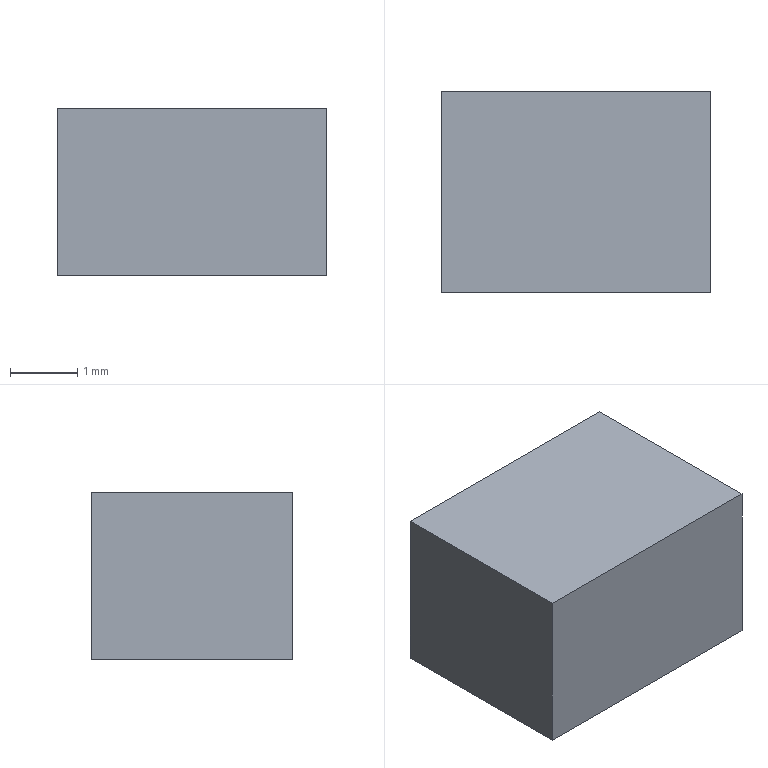Part | Creo | 1 solid | 6 faces | box 4 x 3 x 2.5 mm | volume 30 mm3 | plane 6
STEP:
#1=CARTESIAN_POINT('',(0.,0.,0.));
#2=DIRECTION('',(0.,0.,1.));
#3=DIRECTION('',(1.,0.,0.));
#4=AXIS2_PLACEMENT_3D('',#1,#2,#3);
#5=CARTESIAN_POINT('',(3.25,-1.5,0.));
#6=VERTEX_POINT('',#5);
#7=CARTESIAN_POINT('',(-0.75,-1.5,0.));
#8=VERTEX_POINT('',#7);
#9=CARTESIAN_POINT('',(3.25,-1.5,0.));
#10=DIRECTION('',(-1.,0.,0.));
#11=VECTOR('',#10,4.);
#12=LINE('',#9,#11);
#13=EDGE_CURVE('',#6,#8,#12,.T.);
#14=ORIENTED_EDGE('',*,*,#13,.F.);
#15=CARTESIAN_POINT('',(3.25,1.5,0.));
#16=VERTEX_POINT('',#15);
#17=CARTESIAN_POINT('',(3.25,1.5,0.));
#18=DIRECTION('',(0.,-1.,0.));
#19=VECTOR('',#18,3.);
#20=LINE('',#17,#19);
#21=EDGE_CURVE('',#16,#6,#20,.T.);
#22=ORIENTED_EDGE('',*,*,#21,.F.);
#23=CARTESIAN_POINT('',(-0.75,1.5,0.));
#24=VERTEX_POINT('',#23);
#25=CARTESIAN_POINT('',(-0.75,1.5,0.));
#26=DIRECTION('',(1.,0.,0.));
#27=VECTOR('',#26,4.);
#28=LINE('',#25,#27);
#29=EDGE_CURVE('',#24,#16,#28,.T.);
#30=ORIENTED_EDGE('',*,*,#29,.F.);
#31=CARTESIAN_POINT('',(-0.75,-1.5,0.));
#32=DIRECTION('',(0.,1.,0.));
#33=VECTOR('',#32,3.);
#34=LINE('',#31,#33);
#35=EDGE_CURVE('',#8,#24,#34,.T.);
#36=ORIENTED_EDGE('',*,*,#35,.F.);
#37=EDGE_LOOP('',(#14,#22,#30,#36));
#38=FACE_OUTER_BOUND('',#37,.F.);
#39=CARTESIAN_POINT('',(0.,0.,0.));
#40=DIRECTION('',(0.,0.,1.));
#41=DIRECTION('',(1.,0.,0.));
#42=AXIS2_PLACEMENT_3D('',#39,#40,#41);
#43=PLANE('',#42);
#44=ADVANCED_FACE('',(#38),#43,.F.);
#45=ORIENTED_EDGE('',*,*,#13,.T.);
#46=CARTESIAN_POINT('',(-0.75,-1.5,2.5));
#47=VERTEX_POINT('',#46);
#48=CARTESIAN_POINT('',(-0.75,-1.5,2.5));
#49=DIRECTION('',(0.,0.,-1.));
#50=VECTOR('',#49,2.5);
#51=LINE('',#48,#50);
#52=EDGE_CURVE('',#47,#8,#51,.T.);
#53=ORIENTED_EDGE('',*,*,#52,.F.);
#54=CARTESIAN_POINT('',(3.25,-1.5,2.5));
#55=VERTEX_POINT('',#54);
#56=CARTESIAN_POINT('',(3.25,-1.5,2.5));
#57=DIRECTION('',(-1.,0.,0.));
#58=VECTOR('',#57,4.);
#59=LINE('',#56,#58);
#60=EDGE_CURVE('',#55,#47,#59,.T.);
#61=ORIENTED_EDGE('',*,*,#60,.F.);
#62=CARTESIAN_POINT('',(3.25,-1.5,2.5));
#63=DIRECTION('',(0.,0.,-1.));
#64=VECTOR('',#63,2.5);
#65=LINE('',#62,#64);
#66=EDGE_CURVE('',#55,#6,#65,.T.);
#67=ORIENTED_EDGE('',*,*,#66,.T.);
#68=EDGE_LOOP('',(#45,#53,#61,#67));
#69=FACE_OUTER_BOUND('',#68,.F.);
#70=CARTESIAN_POINT('',(-0.75,-1.5,0.));
#71=DIRECTION('',(0.,-1.,0.));
#72=DIRECTION('',(1.,0.,0.));
#73=AXIS2_PLACEMENT_3D('',#70,#71,#72);
#74=PLANE('',#73);
#75=ADVANCED_FACE('',(#69),#74,.T.);
#76=ORIENTED_EDGE('',*,*,#35,.T.);
#77=CARTESIAN_POINT('',(-0.75,1.5,2.5));
#78=VERTEX_POINT('',#77);
#79=CARTESIAN_POINT('',(-0.75,1.5,2.5));
#80=DIRECTION('',(0.,0.,-1.));
#81=VECTOR('',#80,2.5);
#82=LINE('',#79,#81);
#83=EDGE_CURVE('',#78,#24,#82,.T.);
#84=ORIENTED_EDGE('',*,*,#83,.F.);
#85=CARTESIAN_POINT('',(-0.75,-1.5,2.5));
#86=DIRECTION('',(0.,1.,0.));
#87=VECTOR('',#86,3.);
#88=LINE('',#85,#87);
#89=EDGE_CURVE('',#47,#78,#88,.T.);
#90=ORIENTED_EDGE('',*,*,#89,.F.);
#91=ORIENTED_EDGE('',*,*,#52,.T.);
#92=EDGE_LOOP('',(#76,#84,#90,#91));
#93=FACE_OUTER_BOUND('',#92,.F.);
#94=CARTESIAN_POINT('',(-0.75,1.5,0.));
#95=DIRECTION('',(-1.,0.,0.));
#96=DIRECTION('',(0.,-1.,0.));
#97=AXIS2_PLACEMENT_3D('',#94,#95,#96);
#98=PLANE('',#97);
#99=ADVANCED_FACE('',(#93),#98,.T.);
#100=ORIENTED_EDGE('',*,*,#29,.T.);
#101=CARTESIAN_POINT('',(3.25,1.5,2.5));
#102=VERTEX_POINT('',#101);
#103=CARTESIAN_POINT('',(3.25,1.5,2.5));
#104=DIRECTION('',(0.,0.,-1.));
#105=VECTOR('',#104,2.5);
#106=LINE('',#103,#105);
#107=EDGE_CURVE('',#102,#16,#106,.T.);
#108=ORIENTED_EDGE('',*,*,#107,.F.);
#109=CARTESIAN_POINT('',(-0.75,1.5,2.5));
#110=DIRECTION('',(1.,0.,0.));
#111=VECTOR('',#110,4.);
#112=LINE('',#109,#111);
#113=EDGE_CURVE('',#78,#102,#112,.T.);
#114=ORIENTED_EDGE('',*,*,#113,.F.);
#115=ORIENTED_EDGE('',*,*,#83,.T.);
#116=EDGE_LOOP('',(#100,#108,#114,#115));
#117=FACE_OUTER_BOUND('',#116,.F.);
#118=CARTESIAN_POINT('',(3.25,1.5,0.));
#119=DIRECTION('',(0.,1.,0.));
#120=DIRECTION('',(-1.,0.,0.));
#121=AXIS2_PLACEMENT_3D('',#118,#119,#120);
#122=PLANE('',#121);
#123=ADVANCED_FACE('',(#117),#122,.T.);
#124=ORIENTED_EDGE('',*,*,#21,.T.);
#125=ORIENTED_EDGE('',*,*,#66,.F.);
#126=CARTESIAN_POINT('',(3.25,1.5,2.5));
#127=DIRECTION('',(0.,-1.,0.));
#128=VECTOR('',#127,3.);
#129=LINE('',#126,#128);
#130=EDGE_CURVE('',#102,#55,#129,.T.);
#131=ORIENTED_EDGE('',*,*,#130,.F.);
#132=ORIENTED_EDGE('',*,*,#107,.T.);
#133=EDGE_LOOP('',(#124,#125,#131,#132));
#134=FACE_OUTER_BOUND('',#133,.F.);
#135=CARTESIAN_POINT('',(3.25,-1.5,0.));
#136=DIRECTION('',(1.,0.,0.));
#137=DIRECTION('',(0.,1.,0.));
#138=AXIS2_PLACEMENT_3D('',#135,#136,#137);
#139=PLANE('',#138);
#140=ADVANCED_FACE('',(#134),#139,.T.);
#141=ORIENTED_EDGE('',*,*,#60,.T.);
#142=ORIENTED_EDGE('',*,*,#89,.T.);
#143=ORIENTED_EDGE('',*,*,#113,.T.);
#144=ORIENTED_EDGE('',*,*,#130,.T.);
#145=EDGE_LOOP('',(#141,#142,#143,#144));
#146=FACE_OUTER_BOUND('',#145,.F.);
#147=CARTESIAN_POINT('',(0.,0.,2.5));
#148=DIRECTION('',(0.,0.,1.));
#149=DIRECTION('',(1.,0.,0.));
#150=AXIS2_PLACEMENT_3D('',#147,#148,#149);
#151=PLANE('',#150);
#152=ADVANCED_FACE('',(#146),#151,.T.);
#153=CLOSED_SHELL('',(#44,#75,#99,#123,#140,#152));
#154=MANIFOLD_SOLID_BREP('',#153);
#155=(LENGTH_UNIT()NAMED_UNIT(*)SI_UNIT(.MILLI.,.METRE.));
#156=UNCERTAINTY_MEASURE_WITH_UNIT(LENGTH_MEASURE(0.000559),#155,'','');
#157=(NAMED_UNIT(*)PLANE_ANGLE_UNIT()SI_UNIT($,.RADIAN.));
#158=PLANE_ANGLE_MEASURE_WITH_UNIT(PLANE_ANGLE_MEASURE(0.01745),#157);
#159=(CONVERSION_BASED_UNIT('DEGREE',#158)NAMED_UNIT(*)PLANE_ANGLE_UNIT());
#160=(NAMED_UNIT(*)SI_UNIT($,.STERADIAN.)SOLID_ANGLE_UNIT());
#161=(GEOMETRIC_REPRESENTATION_CONTEXT(3)GLOBAL_UNCERTAINTY_ASSIGNED_CONTEXT((#156))GLOBAL_UNIT_ASSIGNED_CONTEXT((#155,#159,#160))REPRESENTATION_CONTEXT('',''));
#162=ADVANCED_BREP_SHAPE_REPRESENTATION('',(#4,#154),#161);